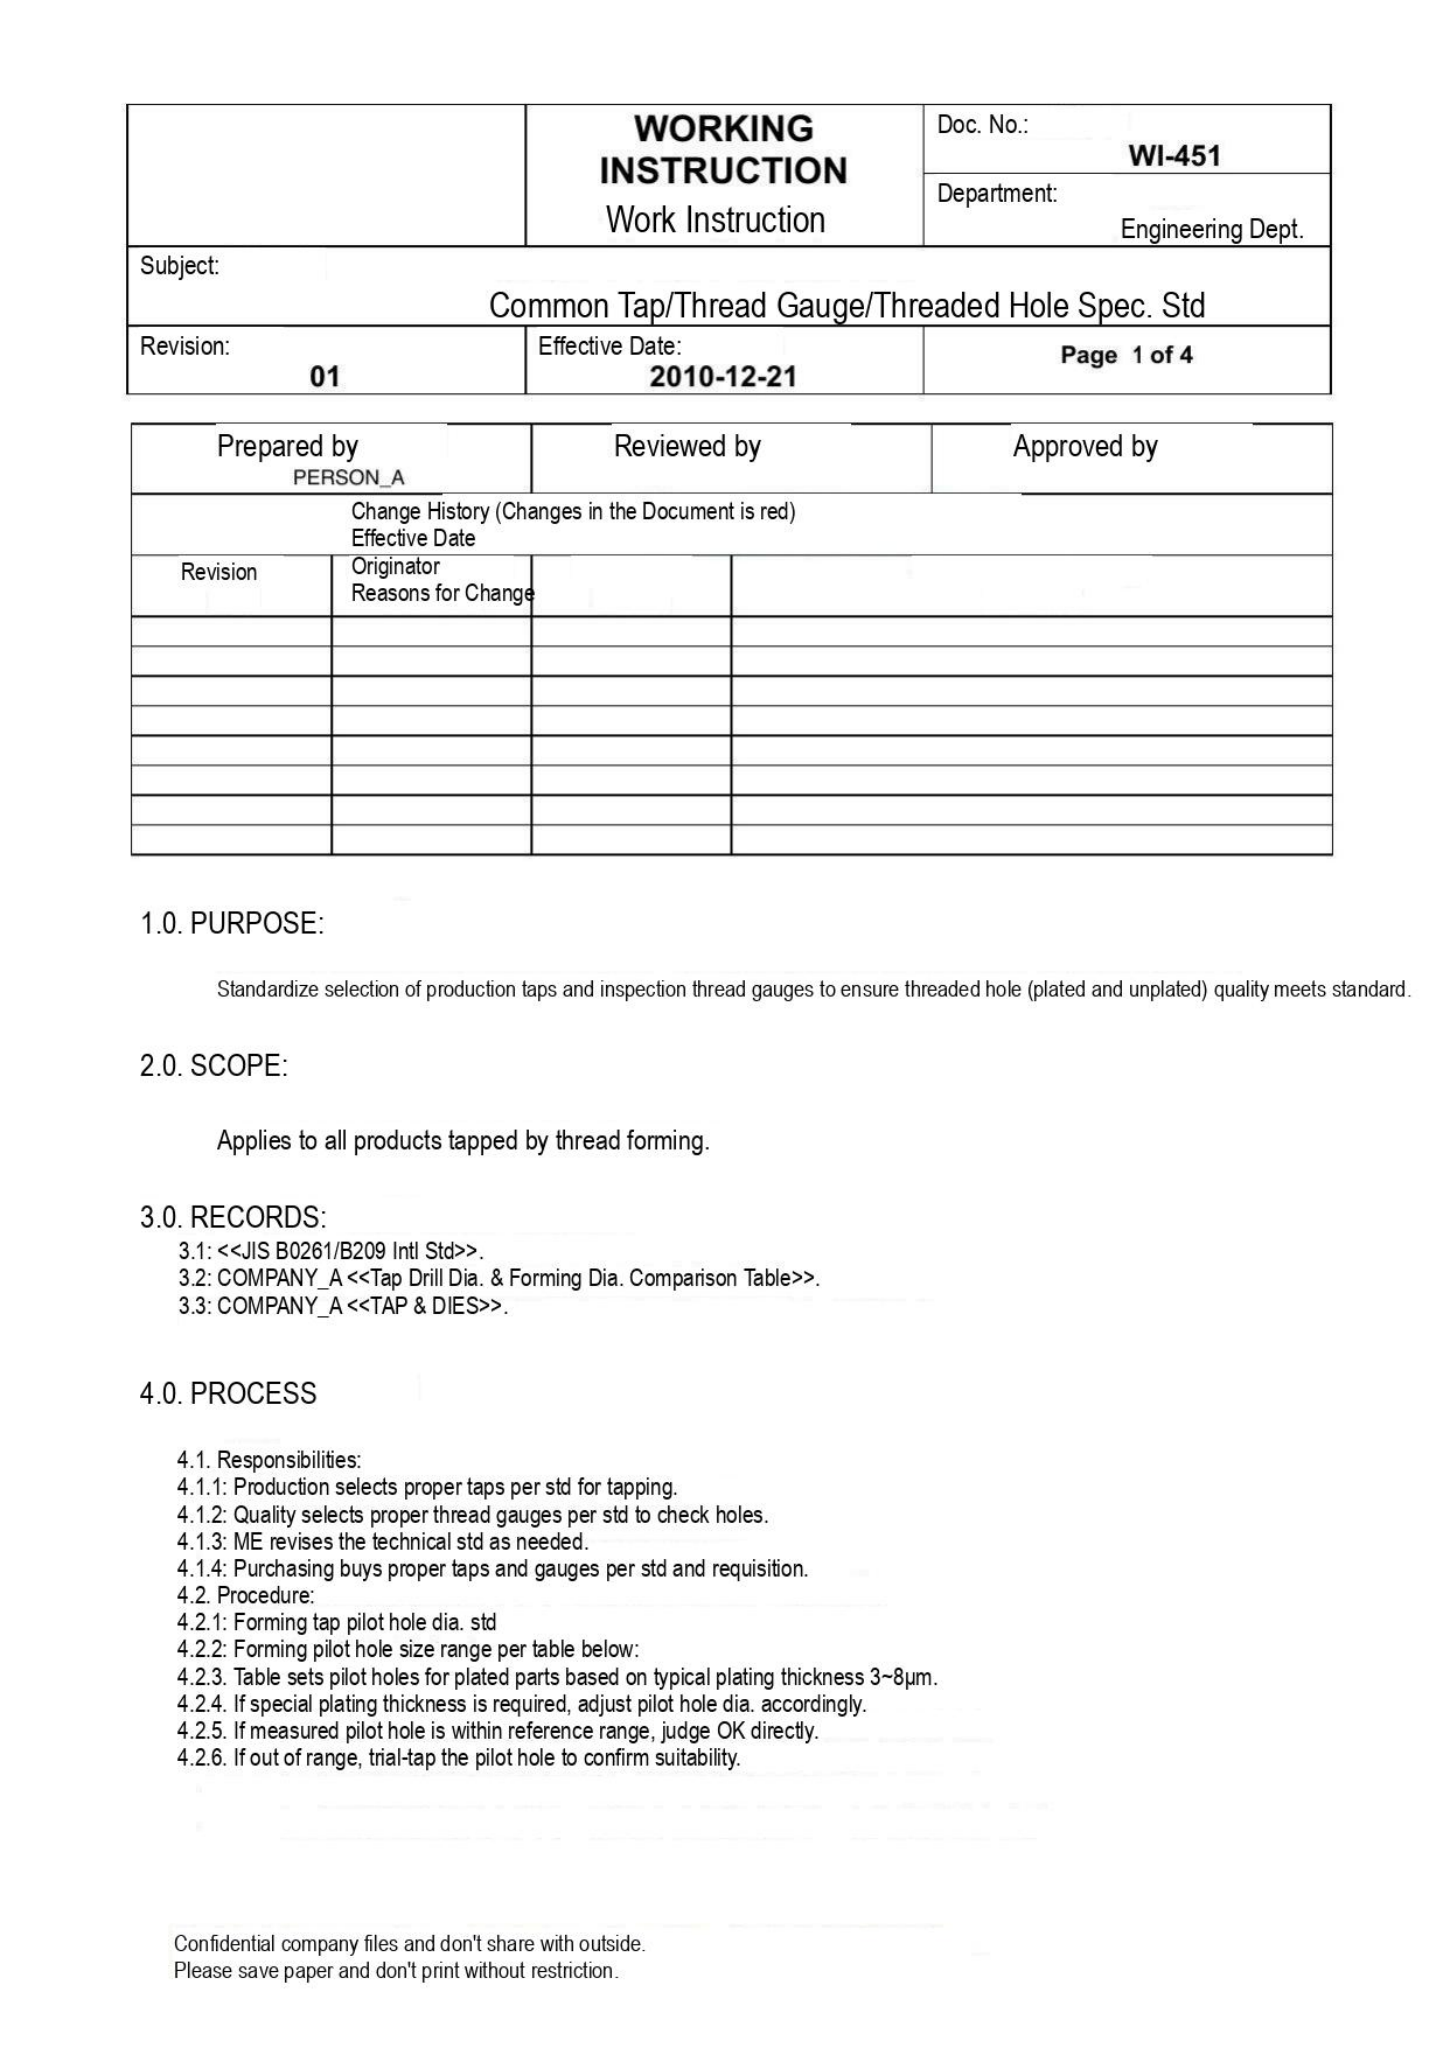| | WORKING INSTRUCTION<br>Work Instruction | Doc. No.: WI-451<br>Department: Engineering Dept. |
|---|---|---|
| Subject: Common Tap/Thread Gauge/Threaded Hole Spec. Std | | |
| Revision: 01 | Effective Date: 2010-12-21 | Page 1 of 4 |

| Prepared by<br>PERSON_A | Reviewed by | Approved by |
|---|---|---|

| Change History (Changes in the Document is red)<br>Effective Date | | | |
|---|---|---|---|
| Revision | Originator<br>Reasons for Change | | |
| | | | |
| | | | |
| | | | |
| | | | |
| | | | |
| | | | |
| | | | |
| | | | |

1.0. PURPOSE:

Standardize selection of production taps and inspection thread gauges to ensure threaded hole (plated and unplated) quality meets standard.

2.0. SCOPE:

Applies to all products tapped by thread forming.

3.0. RECORDS:
3.1: <<JIS B0261/B209 Intl Std>>.
3.2: COMPANY_A <<Tap Drill Dia. & Forming Dia. Comparison Table>>.
3.3: COMPANY_A <<TAP & DIES>>.

4.0. PROCESS

4.1. Responsibilities:
4.1.1: Production selects proper taps per std for tapping.
4.1.2: Quality selects proper thread gauges per std to check holes.
4.1.3: ME revises the technical std as needed.
4.1.4: Purchasing buys proper taps and gauges per std and requisition.
4.2. Procedure:
4.2.1: Forming tap pilot hole dia. std
4.2.2: Forming pilot hole size range per table below:
4.2.3. Table sets pilot holes for plated parts based on typical plating thickness 3~8μm.
4.2.4. If special plating thickness is required, adjust pilot hole dia. accordingly.
4.2.5. If measured pilot hole is within reference range, judge OK directly.
4.2.6. If out of range, trial-tap the pilot hole to confirm suitability.

Confidential company files and don't share with outside.
Please save paper and don't print without restriction.
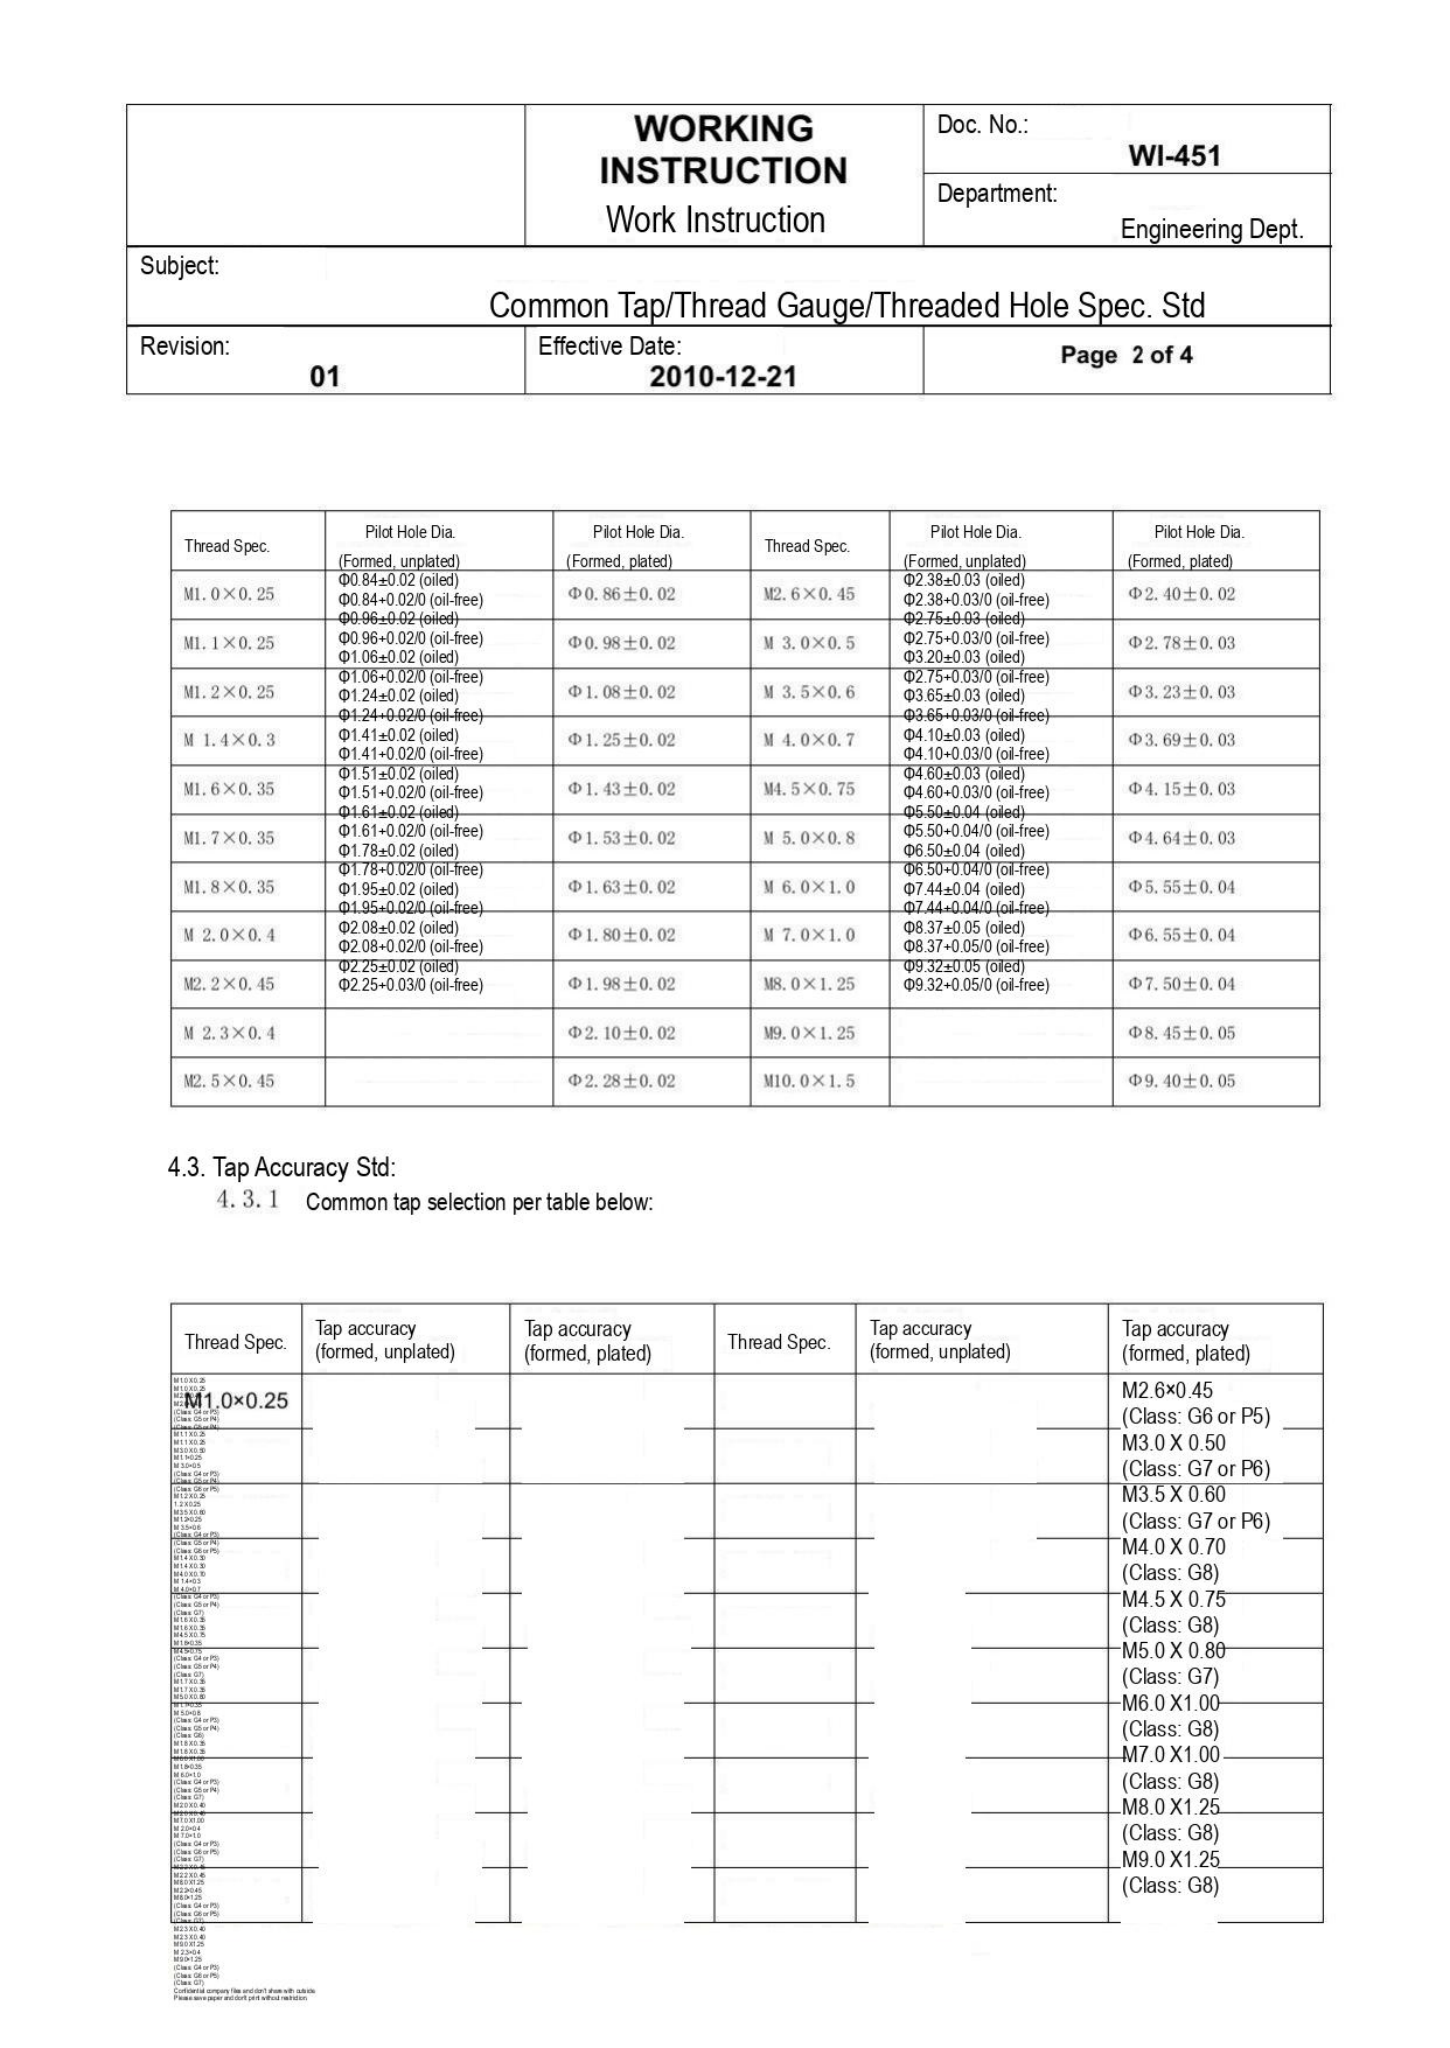| | | WORKING INSTRUCTION<br>Work Instruction | Doc. No.:<br>WI-451<br>Department:<br>Engineering Dept. |
|---|---|---|---|
| Subject:<br>Common Tap/Thread Gauge/Threaded Hole Spec. Std | | | |
| Revision:<br>01 | | Effective Date:<br>2010-12-21 | Page 2 of 4 |

| Thread Spec. | Pilot Hole Dia.<br>(Formed, unplated) | Pilot Hole Dia.<br>(Formed, plated) | Thread Spec. | Pilot Hole Dia.<br>(Formed, unplated) | Pilot Hole Dia.<br>(Formed, plated) |
|---|---|---|---|---|---|
| M1.0×0.25 | Φ0.84±0.02 (oiled)<br>Φ0.84+0.02/0 (oil-free) | Φ0.86±0.02 | M2.6×0.45 | Φ2.38±0.03 (oiled)<br>Φ2.38+0.03/0 (oil-free) | Φ2.40±0.02 |
| M1.1×0.25 | Φ0.96±0.02 (oiled)<br>Φ0.96+0.02/0 (oil-free)<br>Φ1.06±0.02 (oiled) | Φ0.98±0.02 | M 3.0×0.5 | Φ2.75±0.03 (oiled)<br>Φ2.75+0.03/0 (oil-free)<br>Φ3.20±0.03 (oiled) | Φ2.78±0.03 |
| M1.2×0.25 | Φ1.06+0.02/0 (oil-free)<br>Φ1.24±0.02 (oiled) | Φ1.08±0.02 | M 3.5×0.6 | Φ2.75+0.03/0 (oil-free)<br>Φ3.65±0.03 (oiled) | Φ3.23±0.03 |
| M 1.4×0.3 | Φ1.24+0.02/0 (oil-free)<br>Φ1.41±0.02 (oiled)<br>Φ1.41+0.02/0 (oil-free) | Φ1.25±0.02 | M 4.0×0.7 | Φ3.65+0.03/0 (oil-free)<br>Φ4.10±0.03 (oiled)<br>Φ4.10+0.03/0 (oil-free) | Φ3.69±0.03 |
| M1.6×0.35 | Φ1.51±0.02 (oiled)<br>Φ1.51+0.02/0 (oil-free)<br>Φ1.61±0.02 (oiled) | Φ1.43±0.02 | M4.5×0.75 | Φ4.60±0.03 (oiled)<br>Φ4.60+0.03/0 (oil-free)<br>Φ5.50±0.04 (oiled) | Φ4.15±0.03 |
| M1.7×0.35 | Φ1.61+0.02/0 (oil-free)<br>Φ1.78±0.02 (oiled) | Φ1.53±0.02 | M 5.0×0.8 | Φ5.50+0.04/0 (oil-free)<br>Φ6.50±0.04 (oiled) | Φ4.64±0.03 |
| M1.8×0.35 | Φ1.78+0.02/0 (oil-free)<br>Φ1.95±0.02 (oiled)<br>Φ1.95+0.02/0 (oil-free) | Φ1.63±0.02 | M 6.0×1.0 | Φ6.50+0.04/0 (oil-free)<br>Φ7.44±0.04 (oiled)<br>Φ7.44+0.04/0 (oil-free) | Φ5.55±0.04 |
| M 2.0×0.4 | Φ2.08±0.02 (oiled)<br>Φ2.08+0.02/0 (oil-free) | Φ1.80±0.02 | M 7.0×1.0 | Φ8.37±0.05 (oiled)<br>Φ8.37+0.05/0 (oil-free) | Φ6.55±0.04 |
| M2.2×0.45 | Φ2.25±0.02 (oiled)<br>Φ2.25+0.03/0 (oil-free) | Φ1.98±0.02 | M8.0×1.25 | Φ9.32±0.05 (oiled)<br>Φ9.32+0.05/0 (oil-free) | Φ7.50±0.04 |
| M 2.3×0.4 | | Φ2.10±0.02 | M9.0×1.25 | | Φ8.45±0.05 |
| M2.5×0.45 | | Φ2.28±0.02 | M10.0×1.5 | | Φ9.40±0.05 |

4.3. Tap Accuracy Std:

4.3.1 Common tap selection per table below:

| Thread Spec. | Tap accuracy<br>(formed, unplated) | Tap accuracy<br>(formed, plated) | Thread Spec. | Tap accuracy<br>(formed, unplated) | Tap accuracy<br>(formed, plated) |
|---|---|---|---|---|---|
| M1.0×0.25 | | | | | M2.6×0.45<br>(Class: G6 or P5) |
| | | | | | M3.0 X 0.50<br>(Class: G7 or P6) |
| | | | | | M3.5 X 0.60<br>(Class: G7 or P6) |
| | | | | | M4.0 X 0.70<br>(Class: G8) |
| | | | | | M4.5 X 0.75<br>(Class: G8) |
| | | | | | M5.0 X 0.80<br>(Class: G7) |
| | | | | | M6.0 X1.00<br>(Class: G8) |
| | | | | | M7.0 X1.00<br>(Class: G8) |
| | | | | | M8.0 X1.25<br>(Class: G8) |
| | | | | | M9.0 X1.25<br>(Class: G8) |

Confidential company files and don't share with outside
Please save paper and don't print without restriction
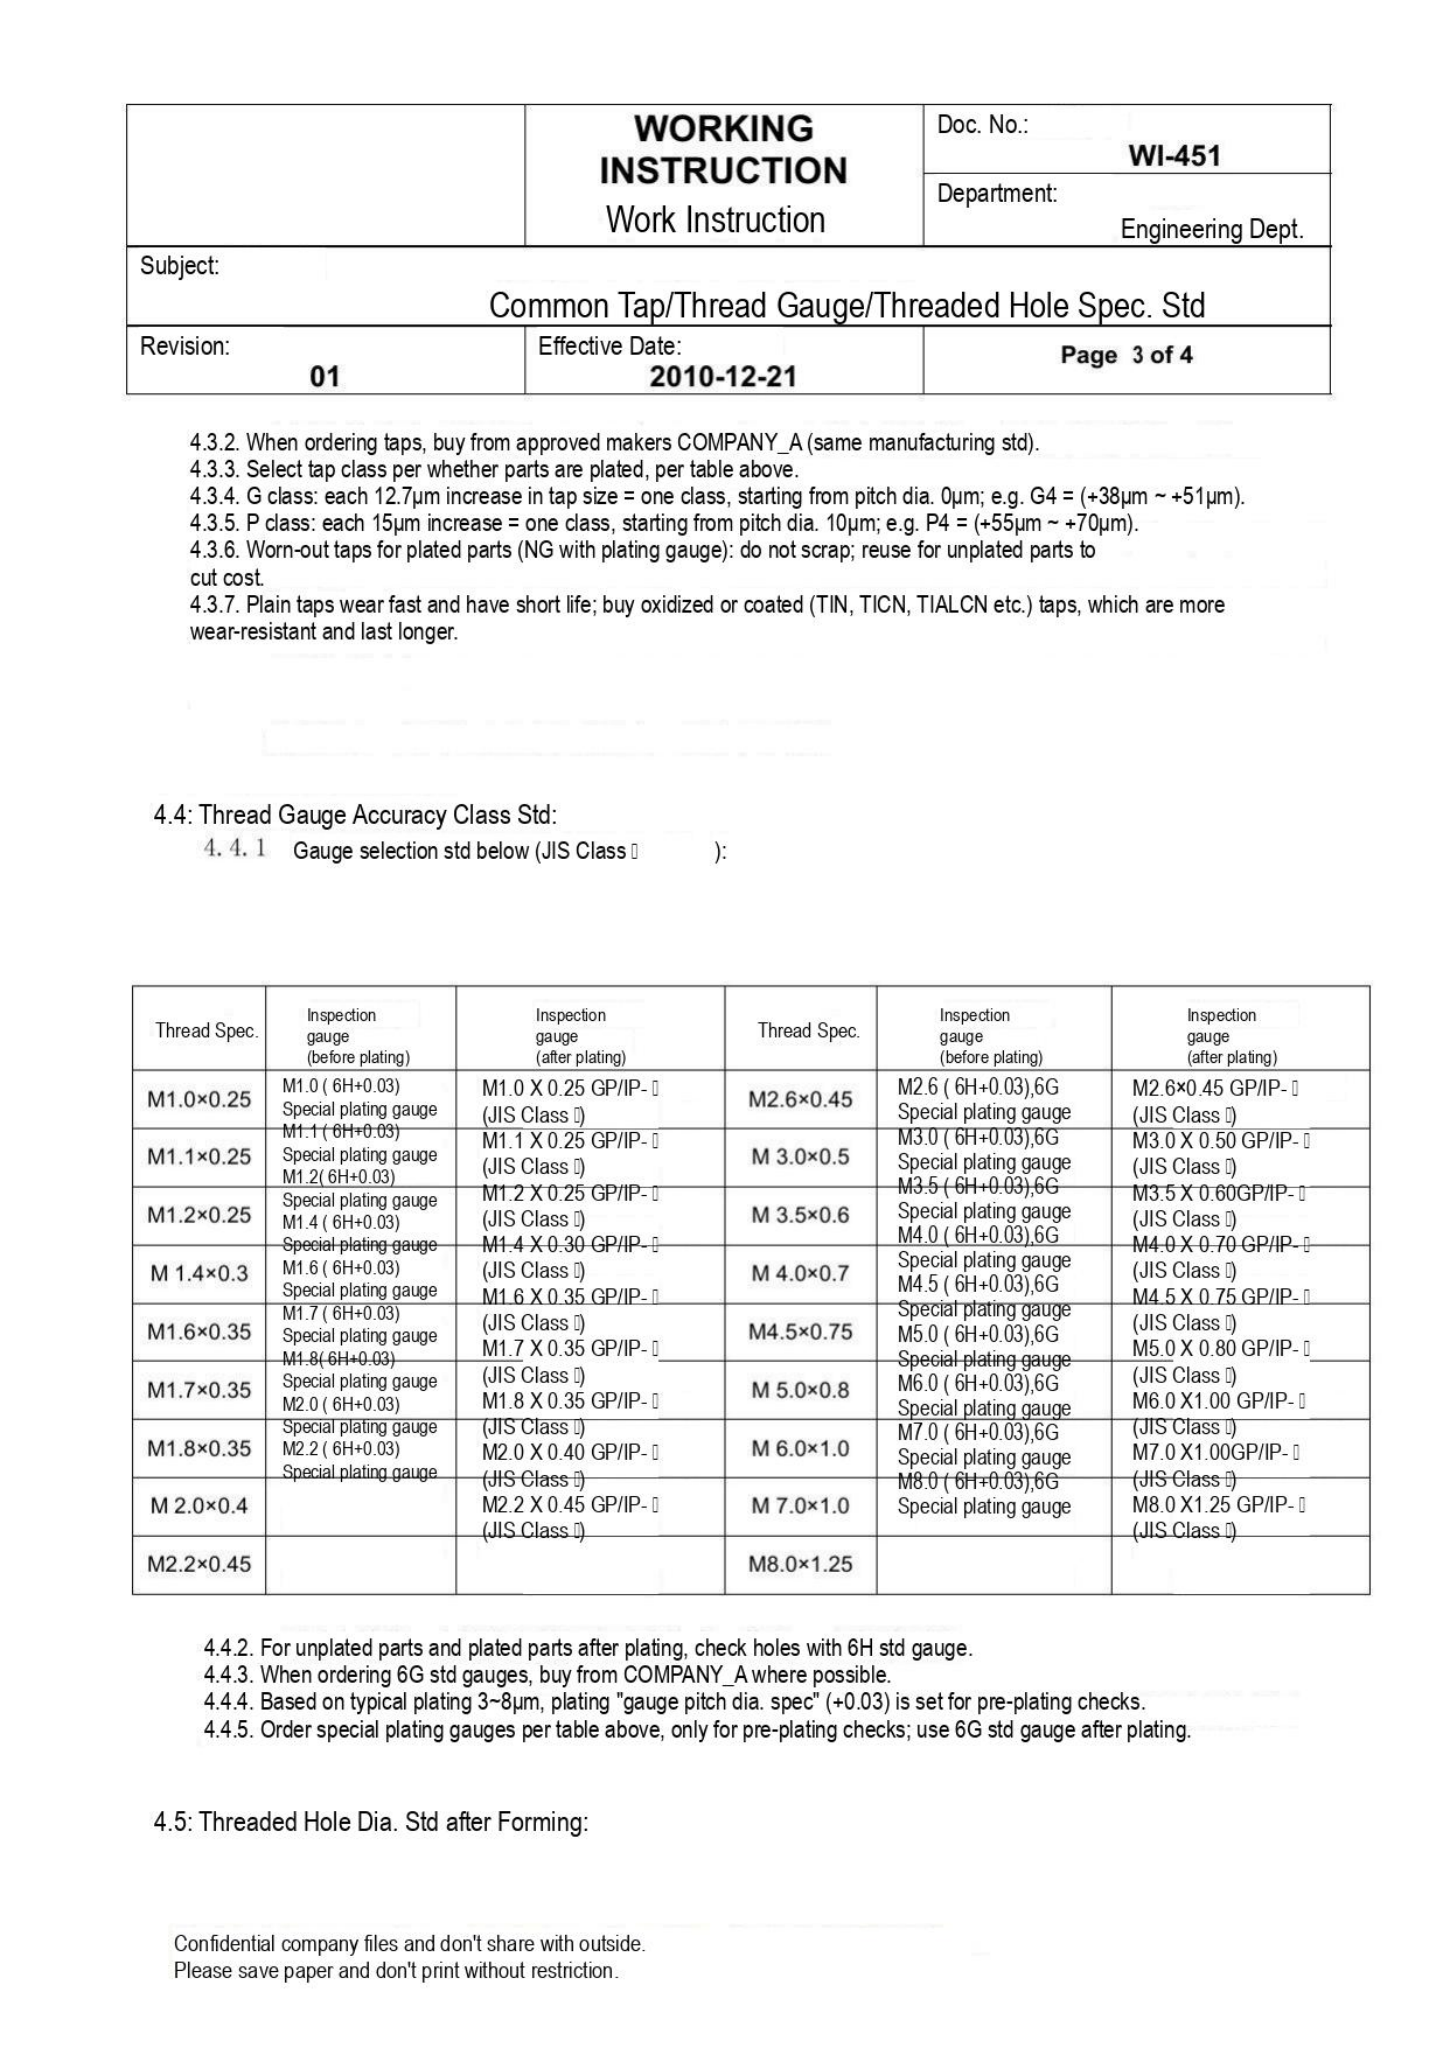| | WORKING INSTRUCTION<br>Work Instruction | Doc. No.: WI-451<br>Department: Engineering Dept. |
|---|---|---|
| Subject: Common Tap/Thread Gauge/Threaded Hole Spec. Std | | |
| Revision: 01 | Effective Date: 2010-12-21 | Page 3 of 4 |

4.3.2. When ordering taps, buy from approved makers COMPANY_A (same manufacturing std).
4.3.3. Select tap class per whether parts are plated, per table above.
4.3.4. G class: each 12.7μm increase in tap size = one class, starting from pitch dia. 0μm; e.g. G4 = (+38μm ~ +51μm).
4.3.5. P class: each 15μm increase = one class, starting from pitch dia. 10μm; e.g. P4 = (+55μm ~ +70μm).
4.3.6. Worn-out taps for plated parts (NG with plating gauge): do not scrap; reuse for unplated parts to cut cost.
4.3.7. Plain taps wear fast and have short life; buy oxidized or coated (TIN, TICN, TIALCN etc.) taps, which are more wear-resistant and last longer.

4.4: Thread Gauge Accuracy Class Std:
4.4.1 Gauge selection std below (JIS Class ):

| Thread Spec. | Inspection gauge (before plating) | Inspection gauge (after plating) | Thread Spec. | Inspection gauge (before plating) | Inspection gauge (after plating) |
|---|---|---|---|---|---|
| M1.0×0.25 | M1.0 ( 6H+0.03) Special plating gauge | M1.0 X 0.25 GP/IP- (JIS Class ) | M2.6×0.45 | M2.6 ( 6H+0.03),6G Special plating gauge | M2.6×0.45 GP/IP- (JIS Class ) |
| M1.1×0.25 | M1.1 ( 6H+0.03) Special plating gauge | M1.1 X 0.25 GP/IP- (JIS Class ) | M 3.0×0.5 | M3.0 ( 6H+0.03),6G Special plating gauge | M3.0 X 0.50 GP/IP- (JIS Class ) |
| M1.2×0.25 | M1.2( 6H+0.03) Special plating gauge | M1.2 X 0.25 GP/IP- (JIS Class ) | M 3.5×0.6 | M3.5 ( 6H+0.03),6G Special plating gauge | M3.5 X 0.60GP/IP- (JIS Class ) |
| M 1.4×0.3 | M1.4 ( 6H+0.03) Special plating gauge | M1.4 X 0.30 GP/IP- (JIS Class ) | M 4.0×0.7 | M4.0 ( 6H+0.03),6G Special plating gauge | M4.0 X 0.70 GP/IP- (JIS Class ) |
| M1.6×0.35 | M1.6 ( 6H+0.03) Special plating gauge | M1.6 X 0.35 GP/IP- (JIS Class ) | M4.5×0.75 | M4.5 ( 6H+0.03),6G Special plating gauge | M4.5 X 0.75 GP/IP- (JIS Class ) |
| M1.7×0.35 | M1.7 ( 6H+0.03) Special plating gauge | M1.7 X 0.35 GP/IP- (JIS Class ) | M 5.0×0.8 | M5.0 ( 6H+0.03),6G Special plating gauge | M5.0 X 0.80 GP/IP- (JIS Class ) |
| M1.8×0.35 | M1.8( 6H+0.03) Special plating gauge | M1.8 X 0.35 GP/IP- (JIS Class ) | M 6.0×1.0 | M6.0 ( 6H+0.03),6G Special plating gauge | M6.0 X1.00 GP/IP- (JIS Class ) |
| M 2.0×0.4 | M2.0 ( 6H+0.03) Special plating gauge | M2.0 X 0.40 GP/IP- (JIS Class ) | M 7.0×1.0 | M7.0 ( 6H+0.03),6G Special plating gauge | M7.0 X1.00GP/IP- (JIS Class ) |
| M2.2×0.45 | M2.2 ( 6H+0.03) Special plating gauge | M2.2 X 0.45 GP/IP- (JIS Class ) | M8.0×1.25 | M8.0 ( 6H+0.03),6G Special plating gauge | M8.0 X1.25 GP/IP- (JIS Class ) |

4.4.2. For unplated parts and plated parts after plating, check holes with 6H std gauge.
4.4.3. When ordering 6G std gauges, buy from COMPANY_A where possible.
4.4.4. Based on typical plating 3~8μm, plating "gauge pitch dia. spec" (+0.03) is set for pre-plating checks.
4.4.5. Order special plating gauges per table above, only for pre-plating checks; use 6G std gauge after plating.

4.5: Threaded Hole Dia. Std after Forming:

Confidential company files and don't share with outside.
Please save paper and don't print without restriction.
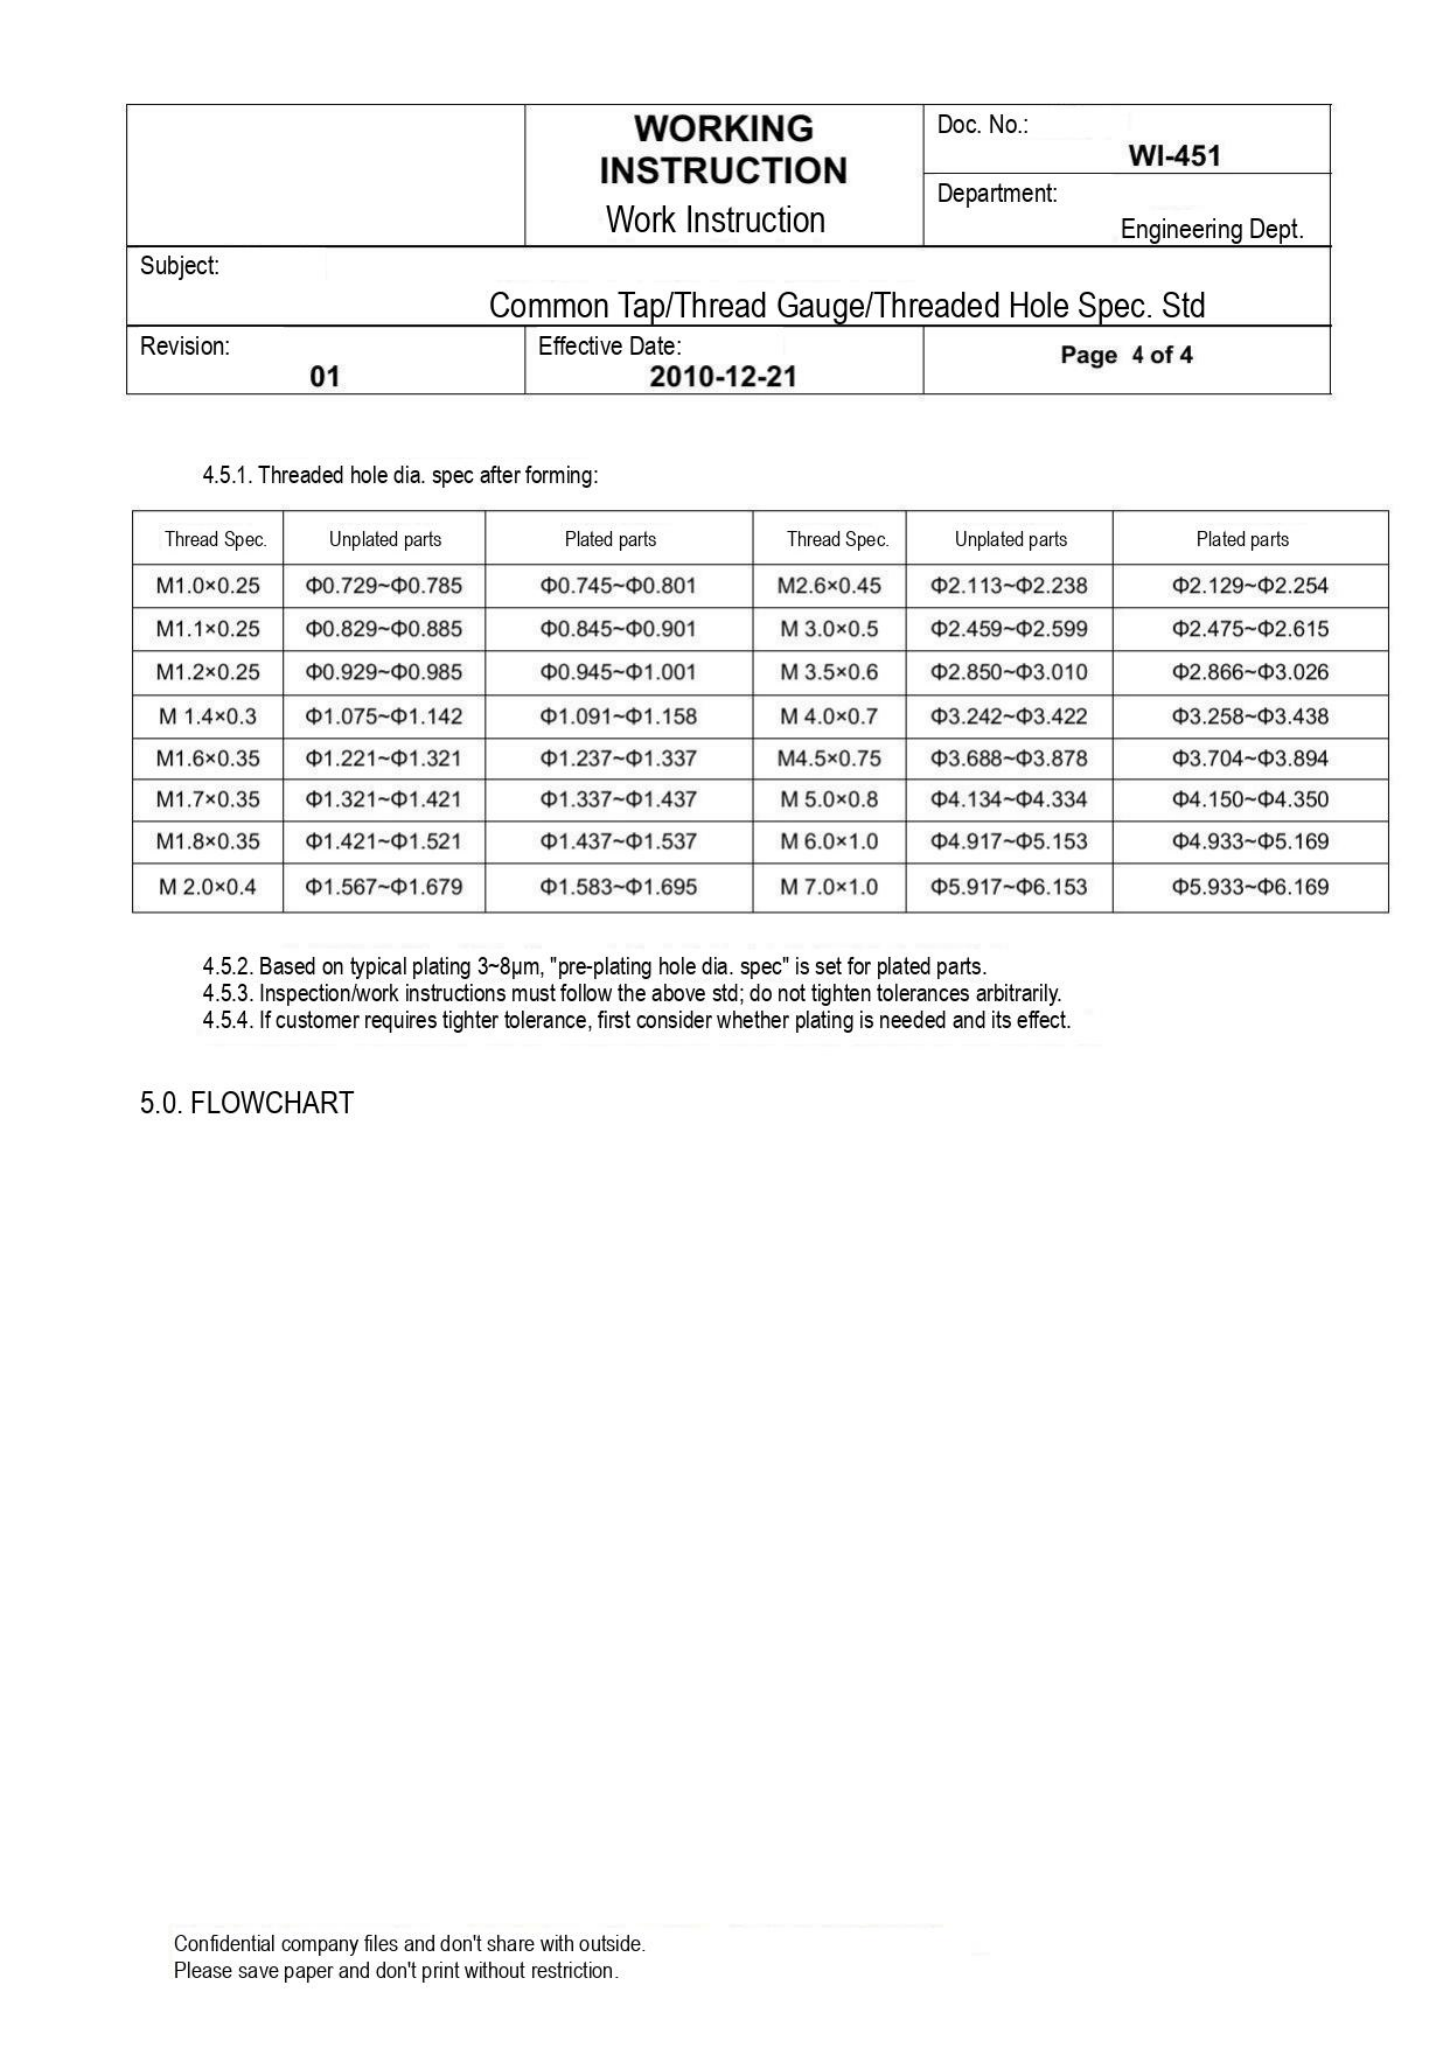| | WORKING INSTRUCTION<br>Work Instruction | Doc. No.: WI-451<br>Department: Engineering Dept. |
|---|---|---|
| Subject: Common Tap/Thread Gauge/Threaded Hole Spec. Std | | |
| Revision: 01 | Effective Date: 2010-12-21 | Page 4 of 4 |

4.5.1. Threaded hole dia. spec after forming:

| Thread Spec. | Unplated parts | Plated parts | Thread Spec. | Unplated parts | Plated parts |
|---|---|---|---|---|---|
| M1.0×0.25 | Φ0.729~Φ0.785 | Φ0.745~Φ0.801 | M2.6×0.45 | Φ2.113~Φ2.238 | Φ2.129~Φ2.254 |
| M1.1×0.25 | Φ0.829~Φ0.885 | Φ0.845~Φ0.901 | M 3.0×0.5 | Φ2.459~Φ2.599 | Φ2.475~Φ2.615 |
| M1.2×0.25 | Φ0.929~Φ0.985 | Φ0.945~Φ1.001 | M 3.5×0.6 | Φ2.850~Φ3.010 | Φ2.866~Φ3.026 |
| M 1.4×0.3 | Φ1.075~Φ1.142 | Φ1.091~Φ1.158 | M 4.0×0.7 | Φ3.242~Φ3.422 | Φ3.258~Φ3.438 |
| M1.6×0.35 | Φ1.221~Φ1.321 | Φ1.237~Φ1.337 | M4.5×0.75 | Φ3.688~Φ3.878 | Φ3.704~Φ3.894 |
| M1.7×0.35 | Φ1.321~Φ1.421 | Φ1.337~Φ1.437 | M 5.0×0.8 | Φ4.134~Φ4.334 | Φ4.150~Φ4.350 |
| M1.8×0.35 | Φ1.421~Φ1.521 | Φ1.437~Φ1.537 | M 6.0×1.0 | Φ4.917~Φ5.153 | Φ4.933~Φ5.169 |
| M 2.0×0.4 | Φ1.567~Φ1.679 | Φ1.583~Φ1.695 | M 7.0×1.0 | Φ5.917~Φ6.153 | Φ5.933~Φ6.169 |

4.5.2. Based on typical plating 3~8μm, "pre-plating hole dia. spec" is set for plated parts.
4.5.3. Inspection/work instructions must follow the above std; do not tighten tolerances arbitrarily.
4.5.4. If customer requires tighter tolerance, first consider whether plating is needed and its effect.

5.0. FLOWCHART

Confidential company files and don't share with outside.
Please save paper and don't print without restriction.